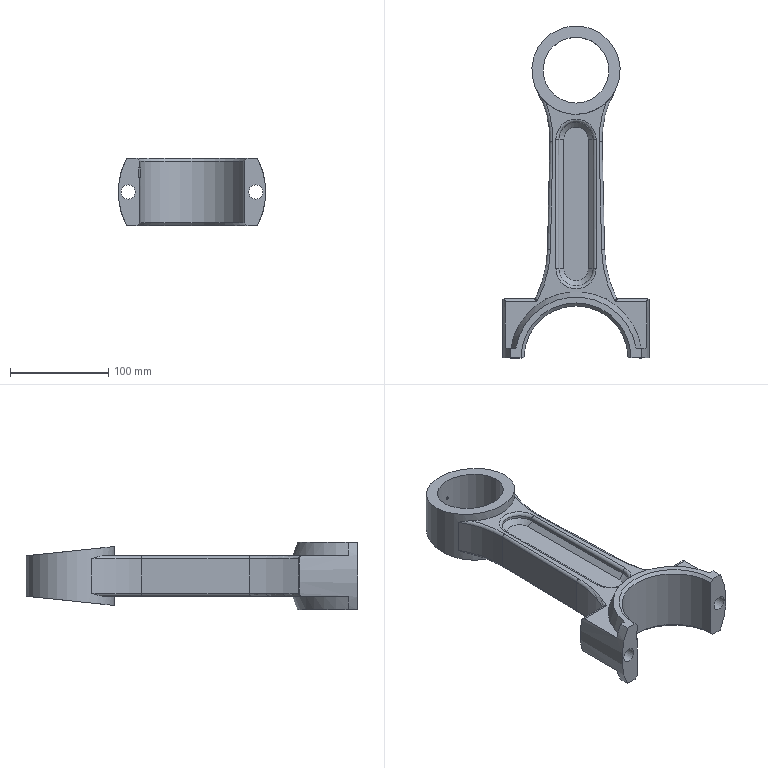Part | NX | features DATUM_CSYS 13, SKETCH 12, EXTRUDE 10, BLEND 6, CHAMFER 6, UNITE 5, DATUM_PLANE 3, SIMPLE HOLE 3, HOLE PACKAGE 2, MIRROR 2, MIRROR_SET 2, SWP104 2, TRIM BODY 1 | 1 solid | 88 faces | box 150 x 338 x 69 mm | volume 706906 mm3 | plane 32 | cylinder 31 | torus 12 | cone 8 | spline 5 | commonest cylinder face diameters 6 x12 35 x4 2 x2 14.5 x2 150 x2 200 x2